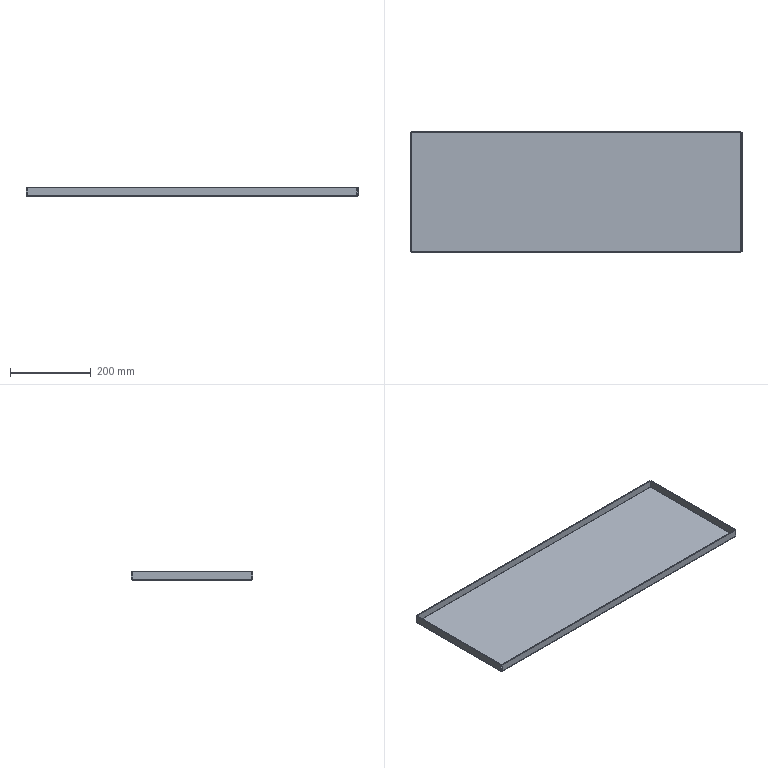Part | STEP file | Part 12 | 1 solid | 38 faces | box 820 x 300 x 20 mm | volume 568950 mm3 | plane 22 | spline 8 | cylinder 8 | commonest cylinder face diameters 1 x4 5 x4
STEP:
#1=CARTESIAN_POINT('',(-407.5,-147.5,-2.));
#2=VERTEX_POINT('',#1);
#3=CARTESIAN_POINT('',(-407.5,147.5,-2.));
#4=VERTEX_POINT('',#3);
#5=CARTESIAN_POINT('',(-407.5,-147.5,-2.));
#6=DIRECTION('',(0.,1.,0.));
#7=VECTOR('',#6,1000.);
#8=LINE('',#5,#7);
#9=EDGE_CURVE('',#2,#4,#8,.T.);
#10=ORIENTED_EDGE('',*,*,#9,.T.);
#11=CARTESIAN_POINT('',(407.5,147.5,-2.));
#12=VERTEX_POINT('',#11);
#13=CARTESIAN_POINT('',(-407.5,147.5,-2.));
#14=DIRECTION('',(1.,0.,0.));
#15=VECTOR('',#14,1000.);
#16=LINE('',#13,#15);
#17=EDGE_CURVE('',#4,#12,#16,.T.);
#18=ORIENTED_EDGE('',*,*,#17,.T.);
#19=CARTESIAN_POINT('',(407.5,-147.5,-2.));
#20=VERTEX_POINT('',#19);
#21=CARTESIAN_POINT('',(407.5,147.5,-2.));
#22=DIRECTION('',(0.,-1.,0.));
#23=VECTOR('',#22,1000.);
#24=LINE('',#21,#23);
#25=EDGE_CURVE('',#12,#20,#24,.T.);
#26=ORIENTED_EDGE('',*,*,#25,.T.);
#27=CARTESIAN_POINT('',(407.5,-147.5,-2.));
#28=DIRECTION('',(-1.,0.,0.));
#29=VECTOR('',#28,1000.);
#30=LINE('',#27,#29);
#31=EDGE_CURVE('',#20,#2,#30,.T.);
#32=ORIENTED_EDGE('',*,*,#31,.T.);
#33=EDGE_LOOP('',(#10,#18,#26,#32));
#34=FACE_OUTER_BOUND('',#33,.T.);
#35=CARTESIAN_POINT('',(0.,0.,-2.));
#36=DIRECTION('',(0.,0.,1.));
#37=DIRECTION('',(1.,0.,0.));
#38=AXIS2_PLACEMENT_3D('',#35,#36,#37);
#39=PLANE('',#38);
#40=ADVANCED_FACE('',(#34),#39,.F.);
#41=CARTESIAN_POINT('',(-407.5,147.5,0.));
#42=VERTEX_POINT('',#41);
#43=CARTESIAN_POINT('',(407.5,147.5,0.));
#44=VERTEX_POINT('',#43);
#45=CARTESIAN_POINT('',(-407.5,147.5,0.));
#46=DIRECTION('',(1.,0.,0.));
#47=VECTOR('',#46,1000.);
#48=LINE('',#45,#47);
#49=EDGE_CURVE('',#42,#44,#48,.T.);
#50=ORIENTED_EDGE('',*,*,#49,.F.);
#51=CARTESIAN_POINT('',(-407.5,-147.5,0.));
#52=VERTEX_POINT('',#51);
#53=CARTESIAN_POINT('',(-407.5,-147.5,0.));
#54=DIRECTION('',(0.,1.,0.));
#55=VECTOR('',#54,1000.);
#56=LINE('',#53,#55);
#57=EDGE_CURVE('',#52,#42,#56,.T.);
#58=ORIENTED_EDGE('',*,*,#57,.F.);
#59=CARTESIAN_POINT('',(407.5,-147.5,0.));
#60=VERTEX_POINT('',#59);
#61=CARTESIAN_POINT('',(407.5,-147.5,0.));
#62=DIRECTION('',(-1.,0.,0.));
#63=VECTOR('',#62,1000.);
#64=LINE('',#61,#63);
#65=EDGE_CURVE('',#60,#52,#64,.T.);
#66=ORIENTED_EDGE('',*,*,#65,.F.);
#67=CARTESIAN_POINT('',(407.5,147.5,0.));
#68=DIRECTION('',(0.,-1.,0.));
#69=VECTOR('',#68,1000.);
#70=LINE('',#67,#69);
#71=EDGE_CURVE('',#44,#60,#70,.T.);
#72=ORIENTED_EDGE('',*,*,#71,.F.);
#73=EDGE_LOOP('',(#50,#58,#66,#72));
#74=FACE_OUTER_BOUND('',#73,.T.);
#75=CARTESIAN_POINT('',(0.,0.,0.));
#76=DIRECTION('',(0.,0.,1.));
#77=DIRECTION('',(1.,0.,0.));
#78=AXIS2_PLACEMENT_3D('',#75,#76,#77);
#79=PLANE('',#78);
#80=ADVANCED_FACE('',(#74),#79,.T.);
#81=CARTESIAN_POINT('',(407.293,150.,0.5));
#82=VERTEX_POINT('',#81);
#83=CARTESIAN_POINT('',(407.293,148.,0.5));
#84=VERTEX_POINT('',#83);
#85=CARTESIAN_POINT('',(407.293,148.,0.5));
#86=DIRECTION('',(0.,-1.,0.));
#87=VECTOR('',#86,1000.);
#88=LINE('',#85,#87);
#89=EDGE_CURVE('',#82,#84,#88,.T.);
#90=ORIENTED_EDGE('',*,*,#89,.T.);
#91=CARTESIAN_POINT('',(407.5,147.5,0.));
#92=CARTESIAN_POINT('',(407.465,147.631,0.));
#93=CARTESIAN_POINT('',(407.431,147.761,0.05389));
#94=CARTESIAN_POINT('',(407.362,147.946,0.239));
#95=CARTESIAN_POINT('',(407.327,148.,0.3691));
#96=CARTESIAN_POINT('',(407.293,148.,0.5));
#97=B_SPLINE_CURVE_WITH_KNOTS('',3,(#91,#92,#93,#94,#95,#96),.UNSPECIFIED.,.F.,.F.,(4,2,4),(0.,0.5,1.),.UNSPECIFIED.);
#98=EDGE_CURVE('',#44,#84,#97,.T.);
#99=ORIENTED_EDGE('',*,*,#98,.F.);
#100=CARTESIAN_POINT('',(407.5,147.5,0.));
#101=DIRECTION('',(0.,0.,-1.));
#102=VECTOR('',#101,1000.);
#103=LINE('',#100,#102);
#104=EDGE_CURVE('',#44,#12,#103,.T.);
#105=ORIENTED_EDGE('',*,*,#104,.T.);
#106=CARTESIAN_POINT('',(407.5,147.5,-2.));
#107=CARTESIAN_POINT('',(407.483,147.827,-2.));
#108=CARTESIAN_POINT('',(407.465,148.154,-1.935));
#109=CARTESIAN_POINT('',(407.431,148.759,-1.684));
#110=CARTESIAN_POINT('',(407.414,149.036,-1.499));
#111=CARTESIAN_POINT('',(407.379,149.499,-1.036));
#112=CARTESIAN_POINT('',(407.362,149.684,-0.759));
#113=CARTESIAN_POINT('',(407.327,149.935,-0.1544));
#114=CARTESIAN_POINT('',(407.31,150.,0.1728));
#115=CARTESIAN_POINT('',(407.293,150.,0.5));
#116=B_SPLINE_CURVE_WITH_KNOTS('',3,(#106,#107,#108,#109,#110,#111,#112,#113,#114,#115),.UNSPECIFIED.,.F.,.F.,(4,2,2,2,4),(0.,0.25,0.5,0.75,1.),.UNSPECIFIED.);
#117=EDGE_CURVE('',#12,#82,#116,.T.);
#118=ORIENTED_EDGE('',*,*,#117,.T.);
#119=EDGE_LOOP('',(#90,#99,#105,#118));
#120=FACE_OUTER_BOUND('',#119,.T.);
#121=CARTESIAN_POINT('',(407.5,147.5,-2.02));
#122=CARTESIAN_POINT('',(407.483,147.83,-2.02));
#123=CARTESIAN_POINT('',(407.465,148.16,-1.954));
#124=CARTESIAN_POINT('',(407.431,148.769,-1.702));
#125=CARTESIAN_POINT('',(407.414,149.049,-1.515));
#126=CARTESIAN_POINT('',(407.379,149.515,-1.049));
#127=CARTESIAN_POINT('',(407.362,149.702,-0.7691));
#128=CARTESIAN_POINT('',(407.327,149.954,-0.1596));
#129=CARTESIAN_POINT('',(407.31,150.02,0.1701));
#130=CARTESIAN_POINT('',(407.293,150.02,0.5));
#131=CARTESIAN_POINT('',(407.5,147.5,-2.));
#132=CARTESIAN_POINT('',(407.483,147.827,-2.));
#133=CARTESIAN_POINT('',(407.465,148.154,-1.935));
#134=CARTESIAN_POINT('',(407.431,148.759,-1.684));
#135=CARTESIAN_POINT('',(407.414,149.036,-1.499));
#136=CARTESIAN_POINT('',(407.379,149.499,-1.036));
#137=CARTESIAN_POINT('',(407.362,149.684,-0.759));
#138=CARTESIAN_POINT('',(407.327,149.935,-0.1544));
#139=CARTESIAN_POINT('',(407.31,150.,0.1727));
#140=CARTESIAN_POINT('',(407.293,150.,0.5));
#141=CARTESIAN_POINT('',(407.5,147.5,0.));
#142=CARTESIAN_POINT('',(407.483,147.565,0.));
#143=CARTESIAN_POINT('',(407.465,147.631,0.01301));
#144=CARTESIAN_POINT('',(407.431,147.752,0.06311));
#145=CARTESIAN_POINT('',(407.414,147.807,0.1002));
#146=CARTESIAN_POINT('',(407.379,147.9,0.1927));
#147=CARTESIAN_POINT('',(407.362,147.937,0.2482));
#148=CARTESIAN_POINT('',(407.327,147.987,0.3691));
#149=CARTESIAN_POINT('',(407.31,148.,0.4345));
#150=CARTESIAN_POINT('',(407.293,148.,0.5));
#151=CARTESIAN_POINT('',(407.5,147.5,0.0202));
#152=CARTESIAN_POINT('',(407.483,147.563,0.0202));
#153=CARTESIAN_POINT('',(407.465,147.626,0.03269));
#154=CARTESIAN_POINT('',(407.431,147.742,0.08076));
#155=CARTESIAN_POINT('',(407.414,147.795,0.1163));
#156=CARTESIAN_POINT('',(407.379,147.884,0.2051));
#157=CARTESIAN_POINT('',(407.362,147.919,0.2584));
#158=CARTESIAN_POINT('',(407.327,147.967,0.3744));
#159=CARTESIAN_POINT('',(407.31,147.98,0.4372));
#160=CARTESIAN_POINT('',(407.293,147.98,0.5));
#161=B_SPLINE_SURFACE_WITH_KNOTS('',1,3,((#121,#122,#123,#124,#125,#126,#127,#128,#129,#130),(#131,#132,#133,#134,#135,#136,#137,#138,#139,#140),(#141,#142,#143,#144,#145,#146,#147,#148,#149,#150),(#151,#152,#153,#154,#155,#156,#157,#158,#159,#160)),.UNSPECIFIED.,.F.,.F.,.F.,(2,1,1,2),(4,2,2,2,4),(-0.01,0.,1.,1.01),(0.,0.25,0.5,0.75,1.),.UNSPECIFIED.);
#162=ADVANCED_FACE('',(#120),#161,.F.);
#163=CARTESIAN_POINT('',(-407.293,148.,0.5));
#164=VERTEX_POINT('',#163);
#165=CARTESIAN_POINT('',(-407.293,148.,0.5));
#166=CARTESIAN_POINT('',(-407.327,148.,0.3691));
#167=CARTESIAN_POINT('',(-407.362,147.946,0.239));
#168=CARTESIAN_POINT('',(-407.431,147.761,0.05389));
#169=CARTESIAN_POINT('',(-407.465,147.631,0.));
#170=CARTESIAN_POINT('',(-407.5,147.5,0.));
#171=B_SPLINE_CURVE_WITH_KNOTS('',3,(#165,#166,#167,#168,#169,#170),.UNSPECIFIED.,.F.,.F.,(4,2,4),(0.,0.5,1.),.UNSPECIFIED.);
#172=EDGE_CURVE('',#164,#42,#171,.T.);
#173=ORIENTED_EDGE('',*,*,#172,.F.);
#174=CARTESIAN_POINT('',(-407.293,150.,0.5));
#175=VERTEX_POINT('',#174);
#176=CARTESIAN_POINT('',(-407.293,148.,0.5));
#177=DIRECTION('',(0.,-1.,0.));
#178=VECTOR('',#177,1000.);
#179=LINE('',#176,#178);
#180=EDGE_CURVE('',#175,#164,#179,.T.);
#181=ORIENTED_EDGE('',*,*,#180,.F.);
#182=CARTESIAN_POINT('',(-407.293,150.,0.5));
#183=CARTESIAN_POINT('',(-407.31,150.,0.1728));
#184=CARTESIAN_POINT('',(-407.327,149.935,-0.1544));
#185=CARTESIAN_POINT('',(-407.362,149.684,-0.759));
#186=CARTESIAN_POINT('',(-407.379,149.499,-1.036));
#187=CARTESIAN_POINT('',(-407.414,149.036,-1.499));
#188=CARTESIAN_POINT('',(-407.431,148.759,-1.684));
#189=CARTESIAN_POINT('',(-407.465,148.154,-1.935));
#190=CARTESIAN_POINT('',(-407.483,147.827,-2.));
#191=CARTESIAN_POINT('',(-407.5,147.5,-2.));
#192=B_SPLINE_CURVE_WITH_KNOTS('',3,(#182,#183,#184,#185,#186,#187,#188,#189,#190,#191),.UNSPECIFIED.,.F.,.F.,(4,2,2,2,4),(0.,0.25,0.5,0.75,1.),.UNSPECIFIED.);
#193=EDGE_CURVE('',#175,#4,#192,.T.);
#194=ORIENTED_EDGE('',*,*,#193,.T.);
#195=CARTESIAN_POINT('',(-407.5,147.5,0.));
#196=DIRECTION('',(0.,0.,-1.));
#197=VECTOR('',#196,1000.);
#198=LINE('',#195,#197);
#199=EDGE_CURVE('',#42,#4,#198,.T.);
#200=ORIENTED_EDGE('',*,*,#199,.F.);
#201=EDGE_LOOP('',(#173,#181,#194,#200));
#202=FACE_OUTER_BOUND('',#201,.T.);
#203=CARTESIAN_POINT('',(-407.293,150.02,0.5));
#204=CARTESIAN_POINT('',(-407.31,150.02,0.1701));
#205=CARTESIAN_POINT('',(-407.327,149.954,-0.1596));
#206=CARTESIAN_POINT('',(-407.362,149.702,-0.7691));
#207=CARTESIAN_POINT('',(-407.379,149.515,-1.049));
#208=CARTESIAN_POINT('',(-407.414,149.049,-1.515));
#209=CARTESIAN_POINT('',(-407.431,148.769,-1.702));
#210=CARTESIAN_POINT('',(-407.465,148.16,-1.954));
#211=CARTESIAN_POINT('',(-407.483,147.83,-2.02));
#212=CARTESIAN_POINT('',(-407.5,147.5,-2.02));
#213=CARTESIAN_POINT('',(-407.293,150.,0.5));
#214=CARTESIAN_POINT('',(-407.31,150.,0.1727));
#215=CARTESIAN_POINT('',(-407.327,149.935,-0.1544));
#216=CARTESIAN_POINT('',(-407.362,149.684,-0.759));
#217=CARTESIAN_POINT('',(-407.379,149.499,-1.036));
#218=CARTESIAN_POINT('',(-407.414,149.036,-1.499));
#219=CARTESIAN_POINT('',(-407.431,148.759,-1.684));
#220=CARTESIAN_POINT('',(-407.465,148.154,-1.935));
#221=CARTESIAN_POINT('',(-407.483,147.827,-2.));
#222=CARTESIAN_POINT('',(-407.5,147.5,-2.));
#223=CARTESIAN_POINT('',(-407.293,148.,0.5));
#224=CARTESIAN_POINT('',(-407.31,148.,0.4345));
#225=CARTESIAN_POINT('',(-407.327,147.987,0.3691));
#226=CARTESIAN_POINT('',(-407.362,147.937,0.2482));
#227=CARTESIAN_POINT('',(-407.379,147.9,0.1927));
#228=CARTESIAN_POINT('',(-407.414,147.807,0.1002));
#229=CARTESIAN_POINT('',(-407.431,147.752,0.06311));
#230=CARTESIAN_POINT('',(-407.465,147.631,0.01301));
#231=CARTESIAN_POINT('',(-407.483,147.565,0.));
#232=CARTESIAN_POINT('',(-407.5,147.5,0.));
#233=CARTESIAN_POINT('',(-407.293,147.98,0.5));
#234=CARTESIAN_POINT('',(-407.31,147.98,0.4372));
#235=CARTESIAN_POINT('',(-407.327,147.967,0.3744));
#236=CARTESIAN_POINT('',(-407.362,147.919,0.2584));
#237=CARTESIAN_POINT('',(-407.379,147.884,0.2051));
#238=CARTESIAN_POINT('',(-407.414,147.795,0.1163));
#239=CARTESIAN_POINT('',(-407.431,147.742,0.08076));
#240=CARTESIAN_POINT('',(-407.465,147.626,0.03269));
#241=CARTESIAN_POINT('',(-407.483,147.563,0.0202));
#242=CARTESIAN_POINT('',(-407.5,147.5,0.0202));
#243=B_SPLINE_SURFACE_WITH_KNOTS('',1,3,((#203,#204,#205,#206,#207,#208,#209,#210,#211,#212),(#213,#214,#215,#216,#217,#218,#219,#220,#221,#222),(#223,#224,#225,#226,#227,#228,#229,#230,#231,#232),(#233,#234,#235,#236,#237,#238,#239,#240,#241,#242)),.UNSPECIFIED.,.F.,.F.,.F.,(2,1,1,2),(4,2,2,2,4),(-0.01,0.,1.,1.01),(0.,0.25,0.5,0.75,1.),.UNSPECIFIED.);
#244=ADVANCED_FACE('',(#202),#243,.F.);
#245=ORIENTED_EDGE('',*,*,#17,.F.);
#246=ORIENTED_EDGE('',*,*,#193,.F.);
#247=CARTESIAN_POINT('',(0.,150.,0.5));
#248=DIRECTION('',(-1.,0.,0.));
#249=VECTOR('',#248,1000.);
#250=LINE('',#247,#249);
#251=EDGE_CURVE('',#82,#175,#250,.T.);
#252=ORIENTED_EDGE('',*,*,#251,.F.);
#253=ORIENTED_EDGE('',*,*,#117,.F.);
#254=EDGE_LOOP('',(#245,#246,#252,#253));
#255=FACE_OUTER_BOUND('',#254,.T.);
#256=CARTESIAN_POINT('',(-407.5,147.5,0.5));
#257=DIRECTION('',(-1.,0.,0.));
#258=DIRECTION('',(0.,1.,0.));
#259=AXIS2_PLACEMENT_3D('',#256,#257,#258);
#260=CYLINDRICAL_SURFACE('',#259,2.5);
#261=ADVANCED_FACE('',(#255),#260,.T.);
#262=ORIENTED_EDGE('',*,*,#49,.T.);
#263=ORIENTED_EDGE('',*,*,#98,.T.);
#264=CARTESIAN_POINT('',(410.,148.,0.5));
#265=DIRECTION('',(-1.,0.,0.));
#266=VECTOR('',#265,1000.);
#267=LINE('',#264,#266);
#268=EDGE_CURVE('',#84,#164,#267,.T.);
#269=ORIENTED_EDGE('',*,*,#268,.T.);
#270=ORIENTED_EDGE('',*,*,#172,.T.);
#271=EDGE_LOOP('',(#262,#263,#269,#270));
#272=FACE_OUTER_BOUND('',#271,.T.);
#273=CARTESIAN_POINT('',(-407.5,147.5,0.5));
#274=DIRECTION('',(-1.,0.,0.));
#275=DIRECTION('',(0.,1.,0.));
#276=AXIS2_PLACEMENT_3D('',#273,#274,#275);
#277=CYLINDRICAL_SURFACE('',#276,0.5);
#278=ADVANCED_FACE('',(#272),#277,.F.);
#279=CARTESIAN_POINT('',(407.293,148.,18.));
#280=VERTEX_POINT('',#279);
#281=CARTESIAN_POINT('',(407.293,150.,18.));
#282=VERTEX_POINT('',#281);
#283=CARTESIAN_POINT('',(407.293,150.,18.));
#284=DIRECTION('',(0.,1.,0.));
#285=VECTOR('',#284,1000.);
#286=LINE('',#283,#285);
#287=EDGE_CURVE('',#280,#282,#286,.T.);
#288=ORIENTED_EDGE('',*,*,#287,.F.);
#289=CARTESIAN_POINT('',(407.293,148.,0.));
#290=DIRECTION('',(0.,0.,1.));
#291=VECTOR('',#290,1000.);
#292=LINE('',#289,#291);
#293=EDGE_CURVE('',#84,#280,#292,.T.);
#294=ORIENTED_EDGE('',*,*,#293,.F.);
#295=ORIENTED_EDGE('',*,*,#89,.F.);
#296=CARTESIAN_POINT('',(407.293,150.,0.));
#297=DIRECTION('',(0.,0.,-1.));
#298=VECTOR('',#297,1000.);
#299=LINE('',#296,#298);
#300=EDGE_CURVE('',#282,#82,#299,.T.);
#301=ORIENTED_EDGE('',*,*,#300,.F.);
#302=EDGE_LOOP('',(#288,#294,#295,#301));
#303=FACE_OUTER_BOUND('',#302,.T.);
#304=CARTESIAN_POINT('',(407.293,148.,0.));
#305=DIRECTION('',(1.,0.,0.));
#306=DIRECTION('',(0.,0.,-1.));
#307=AXIS2_PLACEMENT_3D('',#304,#305,#306);
#308=PLANE('',#307);
#309=ADVANCED_FACE('',(#303),#308,.T.);
#310=CARTESIAN_POINT('',(-407.293,150.,18.));
#311=VERTEX_POINT('',#310);
#312=CARTESIAN_POINT('',(-407.293,150.,0.));
#313=DIRECTION('',(0.,0.,-1.));
#314=VECTOR('',#313,1000.);
#315=LINE('',#312,#314);
#316=EDGE_CURVE('',#311,#175,#315,.T.);
#317=ORIENTED_EDGE('',*,*,#316,.F.);
#318=CARTESIAN_POINT('',(-410.,150.,18.));
#319=DIRECTION('',(-1.,0.,0.));
#320=VECTOR('',#319,1000.);
#321=LINE('',#318,#320);
#322=EDGE_CURVE('',#282,#311,#321,.T.);
#323=ORIENTED_EDGE('',*,*,#322,.F.);
#324=ORIENTED_EDGE('',*,*,#300,.T.);
#325=ORIENTED_EDGE('',*,*,#251,.T.);
#326=EDGE_LOOP('',(#317,#323,#324,#325));
#327=FACE_OUTER_BOUND('',#326,.T.);
#328=CARTESIAN_POINT('',(0.,150.,0.));
#329=DIRECTION('',(0.,1.,0.));
#330=DIRECTION('',(0.,0.,1.));
#331=AXIS2_PLACEMENT_3D('',#328,#329,#330);
#332=PLANE('',#331);
#333=ADVANCED_FACE('',(#327),#332,.T.);
#334=CARTESIAN_POINT('',(-407.293,148.,18.));
#335=VERTEX_POINT('',#334);
#336=CARTESIAN_POINT('',(0.,148.,18.));
#337=DIRECTION('',(-1.,0.,0.));
#338=VECTOR('',#337,1000.);
#339=LINE('',#336,#338);
#340=EDGE_CURVE('',#280,#335,#339,.T.);
#341=ORIENTED_EDGE('',*,*,#340,.T.);
#342=CARTESIAN_POINT('',(-407.293,148.,0.));
#343=DIRECTION('',(0.,0.,1.));
#344=VECTOR('',#343,1000.);
#345=LINE('',#342,#344);
#346=EDGE_CURVE('',#164,#335,#345,.T.);
#347=ORIENTED_EDGE('',*,*,#346,.F.);
#348=ORIENTED_EDGE('',*,*,#268,.F.);
#349=ORIENTED_EDGE('',*,*,#293,.T.);
#350=EDGE_LOOP('',(#341,#347,#348,#349));
#351=FACE_OUTER_BOUND('',#350,.T.);
#352=CARTESIAN_POINT('',(0.,148.,0.));
#353=DIRECTION('',(0.,1.,0.));
#354=DIRECTION('',(0.,0.,1.));
#355=AXIS2_PLACEMENT_3D('',#352,#353,#354);
#356=PLANE('',#355);
#357=ADVANCED_FACE('',(#351),#356,.F.);
#358=CARTESIAN_POINT('',(-407.293,148.,18.));
#359=DIRECTION('',(0.,1.,0.));
#360=VECTOR('',#359,1000.);
#361=LINE('',#358,#360);
#362=EDGE_CURVE('',#335,#311,#361,.T.);
#363=ORIENTED_EDGE('',*,*,#362,.F.);
#364=ORIENTED_EDGE('',*,*,#340,.F.);
#365=ORIENTED_EDGE('',*,*,#287,.T.);
#366=ORIENTED_EDGE('',*,*,#322,.T.);
#367=EDGE_LOOP('',(#363,#364,#365,#366));
#368=FACE_OUTER_BOUND('',#367,.T.);
#369=CARTESIAN_POINT('',(-410.,150.,18.));
#370=DIRECTION('',(0.,0.,1.));
#371=DIRECTION('',(0.,-1.,0.));
#372=AXIS2_PLACEMENT_3D('',#369,#370,#371);
#373=PLANE('',#372);
#374=ADVANCED_FACE('',(#368),#373,.T.);
#375=ORIENTED_EDGE('',*,*,#346,.T.);
#376=ORIENTED_EDGE('',*,*,#362,.T.);
#377=ORIENTED_EDGE('',*,*,#316,.T.);
#378=ORIENTED_EDGE('',*,*,#180,.T.);
#379=EDGE_LOOP('',(#375,#376,#377,#378));
#380=FACE_OUTER_BOUND('',#379,.T.);
#381=CARTESIAN_POINT('',(-407.293,148.,0.));
#382=DIRECTION('',(1.,0.,0.));
#383=DIRECTION('',(0.,0.,-1.));
#384=AXIS2_PLACEMENT_3D('',#381,#382,#383);
#385=PLANE('',#384);
#386=ADVANCED_FACE('',(#380),#385,.F.);
#387=CARTESIAN_POINT('',(410.,-147.293,0.5));
#388=VERTEX_POINT('',#387);
#389=CARTESIAN_POINT('',(408.,-147.293,0.5));
#390=VERTEX_POINT('',#389);
#391=CARTESIAN_POINT('',(408.,-147.293,0.5));
#392=DIRECTION('',(-1.,0.,0.));
#393=VECTOR('',#392,1000.);
#394=LINE('',#391,#393);
#395=EDGE_CURVE('',#388,#390,#394,.T.);
#396=ORIENTED_EDGE('',*,*,#395,.T.);
#397=CARTESIAN_POINT('',(407.5,-147.5,0.));
#398=CARTESIAN_POINT('',(407.631,-147.465,0.));
#399=CARTESIAN_POINT('',(407.761,-147.431,0.05389));
#400=CARTESIAN_POINT('',(407.946,-147.362,0.239));
#401=CARTESIAN_POINT('',(408.,-147.327,0.3691));
#402=CARTESIAN_POINT('',(408.,-147.293,0.5));
#403=B_SPLINE_CURVE_WITH_KNOTS('',3,(#397,#398,#399,#400,#401,#402),.UNSPECIFIED.,.F.,.F.,(4,2,4),(0.,0.5,1.),.UNSPECIFIED.);
#404=EDGE_CURVE('',#60,#390,#403,.T.);
#405=ORIENTED_EDGE('',*,*,#404,.F.);
#406=CARTESIAN_POINT('',(407.5,-147.5,0.));
#407=DIRECTION('',(0.,0.,-1.));
#408=VECTOR('',#407,1000.);
#409=LINE('',#406,#408);
#410=EDGE_CURVE('',#60,#20,#409,.T.);
#411=ORIENTED_EDGE('',*,*,#410,.T.);
#412=CARTESIAN_POINT('',(407.5,-147.5,-2.));
#413=CARTESIAN_POINT('',(407.827,-147.483,-2.));
#414=CARTESIAN_POINT('',(408.154,-147.465,-1.935));
#415=CARTESIAN_POINT('',(408.759,-147.431,-1.684));
#416=CARTESIAN_POINT('',(409.036,-147.414,-1.499));
#417=CARTESIAN_POINT('',(409.499,-147.379,-1.036));
#418=CARTESIAN_POINT('',(409.684,-147.362,-0.759));
#419=CARTESIAN_POINT('',(409.935,-147.327,-0.1544));
#420=CARTESIAN_POINT('',(410.,-147.31,0.1728));
#421=CARTESIAN_POINT('',(410.,-147.293,0.5));
#422=B_SPLINE_CURVE_WITH_KNOTS('',3,(#412,#413,#414,#415,#416,#417,#418,#419,#420,#421),.UNSPECIFIED.,.F.,.F.,(4,2,2,2,4),(0.,0.25,0.5,0.75,1.),.UNSPECIFIED.);
#423=EDGE_CURVE('',#20,#388,#422,.T.);
#424=ORIENTED_EDGE('',*,*,#423,.T.);
#425=EDGE_LOOP('',(#396,#405,#411,#424));
#426=FACE_OUTER_BOUND('',#425,.T.);
#427=CARTESIAN_POINT('',(407.5,-147.5,-2.02));
#428=CARTESIAN_POINT('',(407.83,-147.483,-2.02));
#429=CARTESIAN_POINT('',(408.16,-147.465,-1.954));
#430=CARTESIAN_POINT('',(408.769,-147.431,-1.702));
#431=CARTESIAN_POINT('',(409.049,-147.414,-1.515));
#432=CARTESIAN_POINT('',(409.515,-147.379,-1.049));
#433=CARTESIAN_POINT('',(409.702,-147.362,-0.7691));
#434=CARTESIAN_POINT('',(409.954,-147.327,-0.1596));
#435=CARTESIAN_POINT('',(410.02,-147.31,0.1701));
#436=CARTESIAN_POINT('',(410.02,-147.293,0.5));
#437=CARTESIAN_POINT('',(407.5,-147.5,-2.));
#438=CARTESIAN_POINT('',(407.827,-147.483,-2.));
#439=CARTESIAN_POINT('',(408.154,-147.465,-1.935));
#440=CARTESIAN_POINT('',(408.759,-147.431,-1.684));
#441=CARTESIAN_POINT('',(409.036,-147.414,-1.499));
#442=CARTESIAN_POINT('',(409.499,-147.379,-1.036));
#443=CARTESIAN_POINT('',(409.684,-147.362,-0.759));
#444=CARTESIAN_POINT('',(409.935,-147.327,-0.1544));
#445=CARTESIAN_POINT('',(410.,-147.31,0.1727));
#446=CARTESIAN_POINT('',(410.,-147.293,0.5));
#447=CARTESIAN_POINT('',(407.5,-147.5,0.));
#448=CARTESIAN_POINT('',(407.565,-147.483,0.));
#449=CARTESIAN_POINT('',(407.631,-147.465,0.01301));
#450=CARTESIAN_POINT('',(407.752,-147.431,0.06311));
#451=CARTESIAN_POINT('',(407.807,-147.414,0.1002));
#452=CARTESIAN_POINT('',(407.9,-147.379,0.1927));
#453=CARTESIAN_POINT('',(407.937,-147.362,0.2482));
#454=CARTESIAN_POINT('',(407.987,-147.327,0.3691));
#455=CARTESIAN_POINT('',(408.,-147.31,0.4345));
#456=CARTESIAN_POINT('',(408.,-147.293,0.5));
#457=CARTESIAN_POINT('',(407.5,-147.5,0.0202));
#458=CARTESIAN_POINT('',(407.563,-147.483,0.0202));
#459=CARTESIAN_POINT('',(407.626,-147.465,0.03269));
#460=CARTESIAN_POINT('',(407.742,-147.431,0.08076));
#461=CARTESIAN_POINT('',(407.795,-147.414,0.1163));
#462=CARTESIAN_POINT('',(407.884,-147.379,0.2051));
#463=CARTESIAN_POINT('',(407.919,-147.362,0.2584));
#464=CARTESIAN_POINT('',(407.967,-147.327,0.3744));
#465=CARTESIAN_POINT('',(407.98,-147.31,0.4372));
#466=CARTESIAN_POINT('',(407.98,-147.293,0.5));
#467=B_SPLINE_SURFACE_WITH_KNOTS('',1,3,((#427,#428,#429,#430,#431,#432,#433,#434,#435,#436),(#437,#438,#439,#440,#441,#442,#443,#444,#445,#446),(#447,#448,#449,#450,#451,#452,#453,#454,#455,#456),(#457,#458,#459,#460,#461,#462,#463,#464,#465,#466)),.UNSPECIFIED.,.F.,.F.,.F.,(2,1,1,2),(4,2,2,2,4),(-0.01,0.,1.,1.01),(0.,0.25,0.5,0.75,1.),.UNSPECIFIED.);
#468=ADVANCED_FACE('',(#426),#467,.F.);
#469=CARTESIAN_POINT('',(408.,147.293,0.5));
#470=VERTEX_POINT('',#469);
#471=CARTESIAN_POINT('',(408.,147.293,0.5));
#472=CARTESIAN_POINT('',(408.,147.327,0.3691));
#473=CARTESIAN_POINT('',(407.946,147.362,0.239));
#474=CARTESIAN_POINT('',(407.761,147.431,0.05389));
#475=CARTESIAN_POINT('',(407.631,147.465,0.));
#476=CARTESIAN_POINT('',(407.5,147.5,0.));
#477=B_SPLINE_CURVE_WITH_KNOTS('',3,(#471,#472,#473,#474,#475,#476),.UNSPECIFIED.,.F.,.F.,(4,2,4),(0.,0.5,1.),.UNSPECIFIED.);
#478=EDGE_CURVE('',#470,#44,#477,.T.);
#479=ORIENTED_EDGE('',*,*,#478,.F.);
#480=CARTESIAN_POINT('',(410.,147.293,0.5));
#481=VERTEX_POINT('',#480);
#482=CARTESIAN_POINT('',(408.,147.293,0.5));
#483=DIRECTION('',(-1.,0.,0.));
#484=VECTOR('',#483,1000.);
#485=LINE('',#482,#484);
#486=EDGE_CURVE('',#481,#470,#485,.T.);
#487=ORIENTED_EDGE('',*,*,#486,.F.);
#488=CARTESIAN_POINT('',(410.,147.293,0.5));
#489=CARTESIAN_POINT('',(410.,147.31,0.1728));
#490=CARTESIAN_POINT('',(409.935,147.327,-0.1544));
#491=CARTESIAN_POINT('',(409.684,147.362,-0.759));
#492=CARTESIAN_POINT('',(409.499,147.379,-1.036));
#493=CARTESIAN_POINT('',(409.036,147.414,-1.499));
#494=CARTESIAN_POINT('',(408.759,147.431,-1.684));
#495=CARTESIAN_POINT('',(408.154,147.465,-1.935));
#496=CARTESIAN_POINT('',(407.827,147.483,-2.));
#497=CARTESIAN_POINT('',(407.5,147.5,-2.));
#498=B_SPLINE_CURVE_WITH_KNOTS('',3,(#488,#489,#490,#491,#492,#493,#494,#495,#496,#497),.UNSPECIFIED.,.F.,.F.,(4,2,2,2,4),(0.,0.25,0.5,0.75,1.),.UNSPECIFIED.);
#499=EDGE_CURVE('',#481,#12,#498,.T.);
#500=ORIENTED_EDGE('',*,*,#499,.T.);
#501=ORIENTED_EDGE('',*,*,#104,.F.);
#502=EDGE_LOOP('',(#479,#487,#500,#501));
#503=FACE_OUTER_BOUND('',#502,.T.);
#504=CARTESIAN_POINT('',(410.02,147.293,0.5));
#505=CARTESIAN_POINT('',(410.02,147.31,0.1701));
#506=CARTESIAN_POINT('',(409.954,147.327,-0.1596));
#507=CARTESIAN_POINT('',(409.702,147.362,-0.7691));
#508=CARTESIAN_POINT('',(409.515,147.379,-1.049));
#509=CARTESIAN_POINT('',(409.049,147.414,-1.515));
#510=CARTESIAN_POINT('',(408.769,147.431,-1.702));
#511=CARTESIAN_POINT('',(408.16,147.465,-1.954));
#512=CARTESIAN_POINT('',(407.83,147.483,-2.02));
#513=CARTESIAN_POINT('',(407.5,147.5,-2.02));
#514=CARTESIAN_POINT('',(410.,147.293,0.5));
#515=CARTESIAN_POINT('',(410.,147.31,0.1727));
#516=CARTESIAN_POINT('',(409.935,147.327,-0.1544));
#517=CARTESIAN_POINT('',(409.684,147.362,-0.759));
#518=CARTESIAN_POINT('',(409.499,147.379,-1.036));
#519=CARTESIAN_POINT('',(409.036,147.414,-1.499));
#520=CARTESIAN_POINT('',(408.759,147.431,-1.684));
#521=CARTESIAN_POINT('',(408.154,147.465,-1.935));
#522=CARTESIAN_POINT('',(407.827,147.483,-2.));
#523=CARTESIAN_POINT('',(407.5,147.5,-2.));
#524=CARTESIAN_POINT('',(408.,147.293,0.5));
#525=CARTESIAN_POINT('',(408.,147.31,0.4345));
#526=CARTESIAN_POINT('',(407.987,147.327,0.3691));
#527=CARTESIAN_POINT('',(407.937,147.362,0.2482));
#528=CARTESIAN_POINT('',(407.9,147.379,0.1927));
#529=CARTESIAN_POINT('',(407.807,147.414,0.1002));
#530=CARTESIAN_POINT('',(407.752,147.431,0.06311));
#531=CARTESIAN_POINT('',(407.631,147.465,0.01301));
#532=CARTESIAN_POINT('',(407.565,147.483,0.));
#533=CARTESIAN_POINT('',(407.5,147.5,0.));
#534=CARTESIAN_POINT('',(407.98,147.293,0.5));
#535=CARTESIAN_POINT('',(407.98,147.31,0.4372));
#536=CARTESIAN_POINT('',(407.967,147.327,0.3744));
#537=CARTESIAN_POINT('',(407.919,147.362,0.2584));
#538=CARTESIAN_POINT('',(407.884,147.379,0.2051));
#539=CARTESIAN_POINT('',(407.795,147.414,0.1163));
#540=CARTESIAN_POINT('',(407.742,147.431,0.08076));
#541=CARTESIAN_POINT('',(407.626,147.465,0.03269));
#542=CARTESIAN_POINT('',(407.563,147.483,0.0202));
#543=CARTESIAN_POINT('',(407.5,147.5,0.0202));
#544=B_SPLINE_SURFACE_WITH_KNOTS('',1,3,((#504,#505,#506,#507,#508,#509,#510,#511,#512,#513),(#514,#515,#516,#517,#518,#519,#520,#521,#522,#523),(#524,#525,#526,#527,#528,#529,#530,#531,#532,#533),(#534,#535,#536,#537,#538,#539,#540,#541,#542,#543)),.UNSPECIFIED.,.F.,.F.,.F.,(2,1,1,2),(4,2,2,2,4),(-0.01,0.,1.,1.01),(0.,0.25,0.5,0.75,1.),.UNSPECIFIED.);
#545=ADVANCED_FACE('',(#503),#544,.F.);
#546=ORIENTED_EDGE('',*,*,#25,.F.);
#547=ORIENTED_EDGE('',*,*,#499,.F.);
#548=CARTESIAN_POINT('',(410.,-150.,0.5));
#549=DIRECTION('',(0.,-1.,0.));
#550=VECTOR('',#549,1000.);
#551=LINE('',#548,#550);
#552=EDGE_CURVE('',#481,#388,#551,.T.);
#553=ORIENTED_EDGE('',*,*,#552,.T.);
#554=ORIENTED_EDGE('',*,*,#423,.F.);
#555=EDGE_LOOP('',(#546,#547,#553,#554));
#556=FACE_OUTER_BOUND('',#555,.T.);
#557=CARTESIAN_POINT('',(407.5,147.5,0.5));
#558=DIRECTION('',(0.,1.,0.));
#559=DIRECTION('',(1.,0.,0.));
#560=AXIS2_PLACEMENT_3D('',#557,#558,#559);
#561=CYLINDRICAL_SURFACE('',#560,2.5);
#562=ADVANCED_FACE('',(#556),#561,.T.);
#563=ORIENTED_EDGE('',*,*,#71,.T.);
#564=ORIENTED_EDGE('',*,*,#404,.T.);
#565=CARTESIAN_POINT('',(408.,-150.,0.5));
#566=DIRECTION('',(0.,1.,0.));
#567=VECTOR('',#566,1000.);
#568=LINE('',#565,#567);
#569=EDGE_CURVE('',#390,#470,#568,.T.);
#570=ORIENTED_EDGE('',*,*,#569,.T.);
#571=ORIENTED_EDGE('',*,*,#478,.T.);
#572=EDGE_LOOP('',(#563,#564,#570,#571));
#573=FACE_OUTER_BOUND('',#572,.T.);
#574=CARTESIAN_POINT('',(407.5,147.5,0.5));
#575=DIRECTION('',(0.,1.,0.));
#576=DIRECTION('',(1.,0.,0.));
#577=AXIS2_PLACEMENT_3D('',#574,#575,#576);
#578=CYLINDRICAL_SURFACE('',#577,0.5);
#579=ADVANCED_FACE('',(#573),#578,.F.);
#580=CARTESIAN_POINT('',(408.,-147.293,18.));
#581=VERTEX_POINT('',#580);
#582=CARTESIAN_POINT('',(410.,-147.293,18.));
#583=VERTEX_POINT('',#582);
#584=CARTESIAN_POINT('',(410.,-147.293,18.));
#585=DIRECTION('',(1.,0.,0.));
#586=VECTOR('',#585,1000.);
#587=LINE('',#584,#586);
#588=EDGE_CURVE('',#581,#583,#587,.T.);
#589=ORIENTED_EDGE('',*,*,#588,.F.);
#590=CARTESIAN_POINT('',(408.,-147.293,0.));
#591=DIRECTION('',(0.,0.,1.));
#592=VECTOR('',#591,1000.);
#593=LINE('',#590,#592);
#594=EDGE_CURVE('',#390,#581,#593,.T.);
#595=ORIENTED_EDGE('',*,*,#594,.F.);
#596=ORIENTED_EDGE('',*,*,#395,.F.);
#597=CARTESIAN_POINT('',(410.,-147.293,0.));
#598=DIRECTION('',(0.,0.,1.));
#599=VECTOR('',#598,1000.);
#600=LINE('',#597,#599);
#601=EDGE_CURVE('',#388,#583,#600,.T.);
#602=ORIENTED_EDGE('',*,*,#601,.T.);
#603=EDGE_LOOP('',(#589,#595,#596,#602));
#604=FACE_OUTER_BOUND('',#603,.T.);
#605=CARTESIAN_POINT('',(408.,-147.293,0.));
#606=DIRECTION('',(0.,-1.,0.));
#607=DIRECTION('',(0.,0.,-1.));
#608=AXIS2_PLACEMENT_3D('',#605,#606,#607);
#609=PLANE('',#608);
#610=ADVANCED_FACE('',(#604),#609,.T.);
#611=ORIENTED_EDGE('',*,*,#552,.F.);
#612=CARTESIAN_POINT('',(410.,147.293,18.));
#613=VERTEX_POINT('',#612);
#614=CARTESIAN_POINT('',(410.,147.293,0.));
#615=DIRECTION('',(0.,0.,1.));
#616=VECTOR('',#615,1000.);
#617=LINE('',#614,#616);
#618=EDGE_CURVE('',#481,#613,#617,.T.);
#619=ORIENTED_EDGE('',*,*,#618,.T.);
#620=CARTESIAN_POINT('',(410.,-150.,18.));
#621=DIRECTION('',(0.,1.,0.));
#622=VECTOR('',#621,1000.);
#623=LINE('',#620,#622);
#624=EDGE_CURVE('',#583,#613,#623,.T.);
#625=ORIENTED_EDGE('',*,*,#624,.F.);
#626=ORIENTED_EDGE('',*,*,#601,.F.);
#627=EDGE_LOOP('',(#611,#619,#625,#626));
#628=FACE_OUTER_BOUND('',#627,.T.);
#629=CARTESIAN_POINT('',(410.,0.,0.));
#630=DIRECTION('',(-1.,0.,0.));
#631=DIRECTION('',(0.,0.,1.));
#632=AXIS2_PLACEMENT_3D('',#629,#630,#631);
#633=PLANE('',#632);
#634=ADVANCED_FACE('',(#628),#633,.F.);
#635=CARTESIAN_POINT('',(408.,147.293,18.));
#636=VERTEX_POINT('',#635);
#637=CARTESIAN_POINT('',(408.,147.293,0.));
#638=DIRECTION('',(0.,0.,1.));
#639=VECTOR('',#638,1000.);
#640=LINE('',#637,#639);
#641=EDGE_CURVE('',#470,#636,#640,.T.);
#642=ORIENTED_EDGE('',*,*,#641,.F.);
#643=ORIENTED_EDGE('',*,*,#569,.F.);
#644=ORIENTED_EDGE('',*,*,#594,.T.);
#645=CARTESIAN_POINT('',(408.,0.,18.));
#646=DIRECTION('',(0.,1.,0.));
#647=VECTOR('',#646,1000.);
#648=LINE('',#645,#647);
#649=EDGE_CURVE('',#581,#636,#648,.T.);
#650=ORIENTED_EDGE('',*,*,#649,.T.);
#651=EDGE_LOOP('',(#642,#643,#644,#650));
#652=FACE_OUTER_BOUND('',#651,.T.);
#653=CARTESIAN_POINT('',(408.,0.,0.));
#654=DIRECTION('',(-1.,0.,0.));
#655=DIRECTION('',(0.,0.,1.));
#656=AXIS2_PLACEMENT_3D('',#653,#654,#655);
#657=PLANE('',#656);
#658=ADVANCED_FACE('',(#652),#657,.T.);
#659=CARTESIAN_POINT('',(408.,147.293,18.));
#660=DIRECTION('',(1.,0.,0.));
#661=VECTOR('',#660,1000.);
#662=LINE('',#659,#661);
#663=EDGE_CURVE('',#636,#613,#662,.T.);
#664=ORIENTED_EDGE('',*,*,#663,.F.);
#665=ORIENTED_EDGE('',*,*,#649,.F.);
#666=ORIENTED_EDGE('',*,*,#588,.T.);
#667=ORIENTED_EDGE('',*,*,#624,.T.);
#668=EDGE_LOOP('',(#664,#665,#666,#667));
#669=FACE_OUTER_BOUND('',#668,.T.);
#670=CARTESIAN_POINT('',(410.,-150.,18.));
#671=DIRECTION('',(0.,0.,1.));
#672=DIRECTION('',(1.,0.,0.));
#673=AXIS2_PLACEMENT_3D('',#670,#671,#672);
#674=PLANE('',#673);
#675=ADVANCED_FACE('',(#669),#674,.T.);
#676=ORIENTED_EDGE('',*,*,#641,.T.);
#677=ORIENTED_EDGE('',*,*,#663,.T.);
#678=ORIENTED_EDGE('',*,*,#618,.F.);
#679=ORIENTED_EDGE('',*,*,#486,.T.);
#680=EDGE_LOOP('',(#676,#677,#678,#679));
#681=FACE_OUTER_BOUND('',#680,.T.);
#682=CARTESIAN_POINT('',(408.,147.293,0.));
#683=DIRECTION('',(0.,-1.,0.));
#684=DIRECTION('',(0.,0.,-1.));
#685=AXIS2_PLACEMENT_3D('',#682,#683,#684);
#686=PLANE('',#685);
#687=ADVANCED_FACE('',(#681),#686,.F.);
#688=CARTESIAN_POINT('',(-407.293,-150.,0.5));
#689=VERTEX_POINT('',#688);
#690=CARTESIAN_POINT('',(-407.293,-148.,0.5));
#691=VERTEX_POINT('',#690);
#692=CARTESIAN_POINT('',(-407.293,-148.,0.5));
#693=DIRECTION('',(0.,1.,0.));
#694=VECTOR('',#693,1000.);
#695=LINE('',#692,#694);
#696=EDGE_CURVE('',#689,#691,#695,.T.);
#697=ORIENTED_EDGE('',*,*,#696,.T.);
#698=CARTESIAN_POINT('',(-407.5,-147.5,0.));
#699=CARTESIAN_POINT('',(-407.465,-147.631,0.));
#700=CARTESIAN_POINT('',(-407.431,-147.761,0.05389));
#701=CARTESIAN_POINT('',(-407.362,-147.946,0.239));
#702=CARTESIAN_POINT('',(-407.327,-148.,0.3691));
#703=CARTESIAN_POINT('',(-407.293,-148.,0.5));
#704=B_SPLINE_CURVE_WITH_KNOTS('',3,(#698,#699,#700,#701,#702,#703),.UNSPECIFIED.,.F.,.F.,(4,2,4),(0.,0.5,1.),.UNSPECIFIED.);
#705=EDGE_CURVE('',#52,#691,#704,.T.);
#706=ORIENTED_EDGE('',*,*,#705,.F.);
#707=CARTESIAN_POINT('',(-407.5,-147.5,0.));
#708=DIRECTION('',(0.,0.,-1.));
#709=VECTOR('',#708,1000.);
#710=LINE('',#707,#709);
#711=EDGE_CURVE('',#52,#2,#710,.T.);
#712=ORIENTED_EDGE('',*,*,#711,.T.);
#713=CARTESIAN_POINT('',(-407.5,-147.5,-2.));
#714=CARTESIAN_POINT('',(-407.483,-147.827,-2.));
#715=CARTESIAN_POINT('',(-407.465,-148.154,-1.935));
#716=CARTESIAN_POINT('',(-407.431,-148.759,-1.684));
#717=CARTESIAN_POINT('',(-407.414,-149.036,-1.499));
#718=CARTESIAN_POINT('',(-407.379,-149.499,-1.036));
#719=CARTESIAN_POINT('',(-407.362,-149.684,-0.759));
#720=CARTESIAN_POINT('',(-407.327,-149.935,-0.1544));
#721=CARTESIAN_POINT('',(-407.31,-150.,0.1728));
#722=CARTESIAN_POINT('',(-407.293,-150.,0.5));
#723=B_SPLINE_CURVE_WITH_KNOTS('',3,(#713,#714,#715,#716,#717,#718,#719,#720,#721,#722),.UNSPECIFIED.,.F.,.F.,(4,2,2,2,4),(0.,0.25,0.5,0.75,1.),.UNSPECIFIED.);
#724=EDGE_CURVE('',#2,#689,#723,.T.);
#725=ORIENTED_EDGE('',*,*,#724,.T.);
#726=EDGE_LOOP('',(#697,#706,#712,#725));
#727=FACE_OUTER_BOUND('',#726,.T.);
#728=CARTESIAN_POINT('',(-407.5,-147.5,-2.02));
#729=CARTESIAN_POINT('',(-407.483,-147.83,-2.02));
#730=CARTESIAN_POINT('',(-407.465,-148.16,-1.954));
#731=CARTESIAN_POINT('',(-407.431,-148.769,-1.702));
#732=CARTESIAN_POINT('',(-407.414,-149.049,-1.515));
#733=CARTESIAN_POINT('',(-407.379,-149.515,-1.049));
#734=CARTESIAN_POINT('',(-407.362,-149.702,-0.7691));
#735=CARTESIAN_POINT('',(-407.327,-149.954,-0.1596));
#736=CARTESIAN_POINT('',(-407.31,-150.02,0.1701));
#737=CARTESIAN_POINT('',(-407.293,-150.02,0.5));
#738=CARTESIAN_POINT('',(-407.5,-147.5,-2.));
#739=CARTESIAN_POINT('',(-407.483,-147.827,-2.));
#740=CARTESIAN_POINT('',(-407.465,-148.154,-1.935));
#741=CARTESIAN_POINT('',(-407.431,-148.759,-1.684));
#742=CARTESIAN_POINT('',(-407.414,-149.036,-1.499));
#743=CARTESIAN_POINT('',(-407.379,-149.499,-1.036));
#744=CARTESIAN_POINT('',(-407.362,-149.684,-0.759));
#745=CARTESIAN_POINT('',(-407.327,-149.935,-0.1544));
#746=CARTESIAN_POINT('',(-407.31,-150.,0.1727));
#747=CARTESIAN_POINT('',(-407.293,-150.,0.5));
#748=CARTESIAN_POINT('',(-407.5,-147.5,0.));
#749=CARTESIAN_POINT('',(-407.483,-147.565,0.));
#750=CARTESIAN_POINT('',(-407.465,-147.631,0.01301));
#751=CARTESIAN_POINT('',(-407.431,-147.752,0.06311));
#752=CARTESIAN_POINT('',(-407.414,-147.807,0.1002));
#753=CARTESIAN_POINT('',(-407.379,-147.9,0.1927));
#754=CARTESIAN_POINT('',(-407.362,-147.937,0.2482));
#755=CARTESIAN_POINT('',(-407.327,-147.987,0.3691));
#756=CARTESIAN_POINT('',(-407.31,-148.,0.4345));
#757=CARTESIAN_POINT('',(-407.293,-148.,0.5));
#758=CARTESIAN_POINT('',(-407.5,-147.5,0.0202));
#759=CARTESIAN_POINT('',(-407.483,-147.563,0.0202));
#760=CARTESIAN_POINT('',(-407.465,-147.626,0.03269));
#761=CARTESIAN_POINT('',(-407.431,-147.742,0.08076));
#762=CARTESIAN_POINT('',(-407.414,-147.795,0.1163));
#763=CARTESIAN_POINT('',(-407.379,-147.884,0.2051));
#764=CARTESIAN_POINT('',(-407.362,-147.919,0.2584));
#765=CARTESIAN_POINT('',(-407.327,-147.967,0.3744));
#766=CARTESIAN_POINT('',(-407.31,-147.98,0.4372));
#767=CARTESIAN_POINT('',(-407.293,-147.98,0.5));
#768=B_SPLINE_SURFACE_WITH_KNOTS('',1,3,((#728,#729,#730,#731,#732,#733,#734,#735,#736,#737),(#738,#739,#740,#741,#742,#743,#744,#745,#746,#747),(#748,#749,#750,#751,#752,#753,#754,#755,#756,#757),(#758,#759,#760,#761,#762,#763,#764,#765,#766,#767)),.UNSPECIFIED.,.F.,.F.,.F.,(2,1,1,2),(4,2,2,2,4),(-0.01,0.,1.,1.01),(0.,0.25,0.5,0.75,1.),.UNSPECIFIED.);
#769=ADVANCED_FACE('',(#727),#768,.F.);
#770=CARTESIAN_POINT('',(407.293,-148.,0.5));
#771=VERTEX_POINT('',#770);
#772=CARTESIAN_POINT('',(407.293,-148.,0.5));
#773=CARTESIAN_POINT('',(407.327,-148.,0.3691));
#774=CARTESIAN_POINT('',(407.362,-147.946,0.239));
#775=CARTESIAN_POINT('',(407.431,-147.761,0.05389));
#776=CARTESIAN_POINT('',(407.465,-147.631,0.));
#777=CARTESIAN_POINT('',(407.5,-147.5,0.));
#778=B_SPLINE_CURVE_WITH_KNOTS('',3,(#772,#773,#774,#775,#776,#777),.UNSPECIFIED.,.F.,.F.,(4,2,4),(0.,0.5,1.),.UNSPECIFIED.);
#779=EDGE_CURVE('',#771,#60,#778,.T.);
#780=ORIENTED_EDGE('',*,*,#779,.F.);
#781=CARTESIAN_POINT('',(407.293,-150.,0.5));
#782=VERTEX_POINT('',#781);
#783=CARTESIAN_POINT('',(407.293,-148.,0.5));
#784=DIRECTION('',(0.,1.,0.));
#785=VECTOR('',#784,1000.);
#786=LINE('',#783,#785);
#787=EDGE_CURVE('',#782,#771,#786,.T.);
#788=ORIENTED_EDGE('',*,*,#787,.F.);
#789=CARTESIAN_POINT('',(407.293,-150.,0.5));
#790=CARTESIAN_POINT('',(407.31,-150.,0.1728));
#791=CARTESIAN_POINT('',(407.327,-149.935,-0.1544));
#792=CARTESIAN_POINT('',(407.362,-149.684,-0.759));
#793=CARTESIAN_POINT('',(407.379,-149.499,-1.036));
#794=CARTESIAN_POINT('',(407.414,-149.036,-1.499));
#795=CARTESIAN_POINT('',(407.431,-148.759,-1.684));
#796=CARTESIAN_POINT('',(407.465,-148.154,-1.935));
#797=CARTESIAN_POINT('',(407.483,-147.827,-2.));
#798=CARTESIAN_POINT('',(407.5,-147.5,-2.));
#799=B_SPLINE_CURVE_WITH_KNOTS('',3,(#789,#790,#791,#792,#793,#794,#795,#796,#797,#798),.UNSPECIFIED.,.F.,.F.,(4,2,2,2,4),(0.,0.25,0.5,0.75,1.),.UNSPECIFIED.);
#800=EDGE_CURVE('',#782,#20,#799,.T.);
#801=ORIENTED_EDGE('',*,*,#800,.T.);
#802=ORIENTED_EDGE('',*,*,#410,.F.);
#803=EDGE_LOOP('',(#780,#788,#801,#802));
#804=FACE_OUTER_BOUND('',#803,.T.);
#805=CARTESIAN_POINT('',(407.293,-150.02,0.5));
#806=CARTESIAN_POINT('',(407.31,-150.02,0.1701));
#807=CARTESIAN_POINT('',(407.327,-149.954,-0.1596));
#808=CARTESIAN_POINT('',(407.362,-149.702,-0.7691));
#809=CARTESIAN_POINT('',(407.379,-149.515,-1.049));
#810=CARTESIAN_POINT('',(407.414,-149.049,-1.515));
#811=CARTESIAN_POINT('',(407.431,-148.769,-1.702));
#812=CARTESIAN_POINT('',(407.465,-148.16,-1.954));
#813=CARTESIAN_POINT('',(407.483,-147.83,-2.02));
#814=CARTESIAN_POINT('',(407.5,-147.5,-2.02));
#815=CARTESIAN_POINT('',(407.293,-150.,0.5));
#816=CARTESIAN_POINT('',(407.31,-150.,0.1727));
#817=CARTESIAN_POINT('',(407.327,-149.935,-0.1544));
#818=CARTESIAN_POINT('',(407.362,-149.684,-0.759));
#819=CARTESIAN_POINT('',(407.379,-149.499,-1.036));
#820=CARTESIAN_POINT('',(407.414,-149.036,-1.499));
#821=CARTESIAN_POINT('',(407.431,-148.759,-1.684));
#822=CARTESIAN_POINT('',(407.465,-148.154,-1.935));
#823=CARTESIAN_POINT('',(407.483,-147.827,-2.));
#824=CARTESIAN_POINT('',(407.5,-147.5,-2.));
#825=CARTESIAN_POINT('',(407.293,-148.,0.5));
#826=CARTESIAN_POINT('',(407.31,-148.,0.4345));
#827=CARTESIAN_POINT('',(407.327,-147.987,0.3691));
#828=CARTESIAN_POINT('',(407.362,-147.937,0.2482));
#829=CARTESIAN_POINT('',(407.379,-147.9,0.1927));
#830=CARTESIAN_POINT('',(407.414,-147.807,0.1002));
#831=CARTESIAN_POINT('',(407.431,-147.752,0.06311));
#832=CARTESIAN_POINT('',(407.465,-147.631,0.01301));
#833=CARTESIAN_POINT('',(407.483,-147.565,0.));
#834=CARTESIAN_POINT('',(407.5,-147.5,0.));
#835=CARTESIAN_POINT('',(407.293,-147.98,0.5));
#836=CARTESIAN_POINT('',(407.31,-147.98,0.4372));
#837=CARTESIAN_POINT('',(407.327,-147.967,0.3744));
#838=CARTESIAN_POINT('',(407.362,-147.919,0.2584));
#839=CARTESIAN_POINT('',(407.379,-147.884,0.2051));
#840=CARTESIAN_POINT('',(407.414,-147.795,0.1163));
#841=CARTESIAN_POINT('',(407.431,-147.742,0.08076));
#842=CARTESIAN_POINT('',(407.465,-147.626,0.03269));
#843=CARTESIAN_POINT('',(407.483,-147.563,0.0202));
#844=CARTESIAN_POINT('',(407.5,-147.5,0.0202));
#845=B_SPLINE_SURFACE_WITH_KNOTS('',1,3,((#805,#806,#807,#808,#809,#810,#811,#812,#813,#814),(#815,#816,#817,#818,#819,#820,#821,#822,#823,#824),(#825,#826,#827,#828,#829,#830,#831,#832,#833,#834),(#835,#836,#837,#838,#839,#840,#841,#842,#843,#844)),.UNSPECIFIED.,.F.,.F.,.F.,(2,1,1,2),(4,2,2,2,4),(-0.01,0.,1.,1.01),(0.,0.25,0.5,0.75,1.),.UNSPECIFIED.);
#846=ADVANCED_FACE('',(#804),#845,.F.);
#847=ORIENTED_EDGE('',*,*,#31,.F.);
#848=ORIENTED_EDGE('',*,*,#800,.F.);
#849=CARTESIAN_POINT('',(-410.,-150.,0.5));
#850=DIRECTION('',(-1.,0.,0.));
#851=VECTOR('',#850,1000.);
#852=LINE('',#849,#851);
#853=EDGE_CURVE('',#782,#689,#852,.T.);
#854=ORIENTED_EDGE('',*,*,#853,.T.);
#855=ORIENTED_EDGE('',*,*,#724,.F.);
#856=EDGE_LOOP('',(#847,#848,#854,#855));
#857=FACE_OUTER_BOUND('',#856,.T.);
#858=CARTESIAN_POINT('',(407.5,-147.5,0.5));
#859=DIRECTION('',(1.,0.,0.));
#860=DIRECTION('',(0.,-1.,0.));
#861=AXIS2_PLACEMENT_3D('',#858,#859,#860);
#862=CYLINDRICAL_SURFACE('',#861,2.5);
#863=ADVANCED_FACE('',(#857),#862,.T.);
#864=ORIENTED_EDGE('',*,*,#65,.T.);
#865=ORIENTED_EDGE('',*,*,#705,.T.);
#866=CARTESIAN_POINT('',(-410.,-148.,0.5));
#867=DIRECTION('',(1.,0.,0.));
#868=VECTOR('',#867,1000.);
#869=LINE('',#866,#868);
#870=EDGE_CURVE('',#691,#771,#869,.T.);
#871=ORIENTED_EDGE('',*,*,#870,.T.);
#872=ORIENTED_EDGE('',*,*,#779,.T.);
#873=EDGE_LOOP('',(#864,#865,#871,#872));
#874=FACE_OUTER_BOUND('',#873,.T.);
#875=CARTESIAN_POINT('',(407.5,-147.5,0.5));
#876=DIRECTION('',(1.,0.,0.));
#877=DIRECTION('',(0.,-1.,0.));
#878=AXIS2_PLACEMENT_3D('',#875,#876,#877);
#879=CYLINDRICAL_SURFACE('',#878,0.5);
#880=ADVANCED_FACE('',(#874),#879,.F.);
#881=CARTESIAN_POINT('',(-407.293,-148.,18.));
#882=VERTEX_POINT('',#881);
#883=CARTESIAN_POINT('',(-407.293,-150.,18.));
#884=VERTEX_POINT('',#883);
#885=CARTESIAN_POINT('',(-407.293,-150.,18.));
#886=DIRECTION('',(0.,-1.,0.));
#887=VECTOR('',#886,1000.);
#888=LINE('',#885,#887);
#889=EDGE_CURVE('',#882,#884,#888,.T.);
#890=ORIENTED_EDGE('',*,*,#889,.F.);
#891=CARTESIAN_POINT('',(-407.293,-148.,0.));
#892=DIRECTION('',(0.,0.,1.));
#893=VECTOR('',#892,1000.);
#894=LINE('',#891,#893);
#895=EDGE_CURVE('',#691,#882,#894,.T.);
#896=ORIENTED_EDGE('',*,*,#895,.F.);
#897=ORIENTED_EDGE('',*,*,#696,.F.);
#898=CARTESIAN_POINT('',(-407.293,-150.,0.));
#899=DIRECTION('',(0.,0.,1.));
#900=VECTOR('',#899,1000.);
#901=LINE('',#898,#900);
#902=EDGE_CURVE('',#689,#884,#901,.T.);
#903=ORIENTED_EDGE('',*,*,#902,.T.);
#904=EDGE_LOOP('',(#890,#896,#897,#903));
#905=FACE_OUTER_BOUND('',#904,.T.);
#906=CARTESIAN_POINT('',(-407.293,-148.,0.));
#907=DIRECTION('',(-1.,0.,0.));
#908=DIRECTION('',(0.,0.,1.));
#909=AXIS2_PLACEMENT_3D('',#906,#907,#908);
#910=PLANE('',#909);
#911=ADVANCED_FACE('',(#905),#910,.T.);
#912=ORIENTED_EDGE('',*,*,#853,.F.);
#913=CARTESIAN_POINT('',(407.293,-150.,18.));
#914=VERTEX_POINT('',#913);
#915=CARTESIAN_POINT('',(407.293,-150.,0.));
#916=DIRECTION('',(0.,0.,1.));
#917=VECTOR('',#916,1000.);
#918=LINE('',#915,#917);
#919=EDGE_CURVE('',#782,#914,#918,.T.);
#920=ORIENTED_EDGE('',*,*,#919,.T.);
#921=CARTESIAN_POINT('',(-410.,-150.,18.));
#922=DIRECTION('',(1.,0.,0.));
#923=VECTOR('',#922,1000.);
#924=LINE('',#921,#923);
#925=EDGE_CURVE('',#884,#914,#924,.T.);
#926=ORIENTED_EDGE('',*,*,#925,.F.);
#927=ORIENTED_EDGE('',*,*,#902,.F.);
#928=EDGE_LOOP('',(#912,#920,#926,#927));
#929=FACE_OUTER_BOUND('',#928,.T.);
#930=CARTESIAN_POINT('',(0.,-150.,0.));
#931=DIRECTION('',(0.,1.,0.));
#932=DIRECTION('',(0.,0.,1.));
#933=AXIS2_PLACEMENT_3D('',#930,#931,#932);
#934=PLANE('',#933);
#935=ADVANCED_FACE('',(#929),#934,.F.);
#936=CARTESIAN_POINT('',(407.293,-148.,18.));
#937=VERTEX_POINT('',#936);
#938=CARTESIAN_POINT('',(407.293,-148.,0.));
#939=DIRECTION('',(0.,0.,1.));
#940=VECTOR('',#939,1000.);
#941=LINE('',#938,#940);
#942=EDGE_CURVE('',#771,#937,#941,.T.);
#943=ORIENTED_EDGE('',*,*,#942,.F.);
#944=ORIENTED_EDGE('',*,*,#870,.F.);
#945=ORIENTED_EDGE('',*,*,#895,.T.);
#946=CARTESIAN_POINT('',(0.,-148.,18.));
#947=DIRECTION('',(1.,0.,0.));
#948=VECTOR('',#947,1000.);
#949=LINE('',#946,#948);
#950=EDGE_CURVE('',#882,#937,#949,.T.);
#951=ORIENTED_EDGE('',*,*,#950,.T.);
#952=EDGE_LOOP('',(#943,#944,#945,#951));
#953=FACE_OUTER_BOUND('',#952,.T.);
#954=CARTESIAN_POINT('',(0.,-148.,0.));
#955=DIRECTION('',(0.,1.,0.));
#956=DIRECTION('',(0.,0.,1.));
#957=AXIS2_PLACEMENT_3D('',#954,#955,#956);
#958=PLANE('',#957);
#959=ADVANCED_FACE('',(#953),#958,.T.);
#960=CARTESIAN_POINT('',(407.293,-148.,18.));
#961=DIRECTION('',(0.,-1.,0.));
#962=VECTOR('',#961,1000.);
#963=LINE('',#960,#962);
#964=EDGE_CURVE('',#937,#914,#963,.T.);
#965=ORIENTED_EDGE('',*,*,#964,.F.);
#966=ORIENTED_EDGE('',*,*,#950,.F.);
#967=ORIENTED_EDGE('',*,*,#889,.T.);
#968=ORIENTED_EDGE('',*,*,#925,.T.);
#969=EDGE_LOOP('',(#965,#966,#967,#968));
#970=FACE_OUTER_BOUND('',#969,.T.);
#971=CARTESIAN_POINT('',(-410.,-150.,18.));
#972=DIRECTION('',(0.,0.,1.));
#973=DIRECTION('',(0.,-1.,0.));
#974=AXIS2_PLACEMENT_3D('',#971,#972,#973);
#975=PLANE('',#974);
#976=ADVANCED_FACE('',(#970),#975,.T.);
#977=ORIENTED_EDGE('',*,*,#942,.T.);
#978=ORIENTED_EDGE('',*,*,#964,.T.);
#979=ORIENTED_EDGE('',*,*,#919,.F.);
#980=ORIENTED_EDGE('',*,*,#787,.T.);
#981=EDGE_LOOP('',(#977,#978,#979,#980));
#982=FACE_OUTER_BOUND('',#981,.T.);
#983=CARTESIAN_POINT('',(407.293,-148.,0.));
#984=DIRECTION('',(-1.,0.,0.));
#985=DIRECTION('',(0.,0.,1.));
#986=AXIS2_PLACEMENT_3D('',#983,#984,#985);
#987=PLANE('',#986);
#988=ADVANCED_FACE('',(#982),#987,.F.);
#989=CARTESIAN_POINT('',(-410.,147.293,0.5));
#990=VERTEX_POINT('',#989);
#991=CARTESIAN_POINT('',(-408.,147.293,0.5));
#992=VERTEX_POINT('',#991);
#993=CARTESIAN_POINT('',(-408.,147.293,0.5));
#994=DIRECTION('',(1.,0.,0.));
#995=VECTOR('',#994,1000.);
#996=LINE('',#993,#995);
#997=EDGE_CURVE('',#990,#992,#996,.T.);
#998=ORIENTED_EDGE('',*,*,#997,.T.);
#999=CARTESIAN_POINT('',(-407.5,147.5,0.));
#1000=CARTESIAN_POINT('',(-407.631,147.465,0.));
#1001=CARTESIAN_POINT('',(-407.761,147.431,0.05389));
#1002=CARTESIAN_POINT('',(-407.946,147.362,0.239));
#1003=CARTESIAN_POINT('',(-408.,147.327,0.3691));
#1004=CARTESIAN_POINT('',(-408.,147.293,0.5));
#1005=B_SPLINE_CURVE_WITH_KNOTS('',3,(#999,#1000,#1001,#1002,#1003,#1004),.UNSPECIFIED.,.F.,.F.,(4,2,4),(0.,0.5,1.),.UNSPECIFIED.);
#1006=EDGE_CURVE('',#42,#992,#1005,.T.);
#1007=ORIENTED_EDGE('',*,*,#1006,.F.);
#1008=ORIENTED_EDGE('',*,*,#199,.T.);
#1009=CARTESIAN_POINT('',(-407.5,147.5,-2.));
#1010=CARTESIAN_POINT('',(-407.827,147.483,-2.));
#1011=CARTESIAN_POINT('',(-408.154,147.465,-1.935));
#1012=CARTESIAN_POINT('',(-408.759,147.431,-1.684));
#1013=CARTESIAN_POINT('',(-409.036,147.414,-1.499));
#1014=CARTESIAN_POINT('',(-409.499,147.379,-1.036));
#1015=CARTESIAN_POINT('',(-409.684,147.362,-0.759));
#1016=CARTESIAN_POINT('',(-409.935,147.327,-0.1544));
#1017=CARTESIAN_POINT('',(-410.,147.31,0.1728));
#1018=CARTESIAN_POINT('',(-410.,147.293,0.5));
#1019=B_SPLINE_CURVE_WITH_KNOTS('',3,(#1009,#1010,#1011,#1012,#1013,#1014,#1015,#1016,#1017,#1018),.UNSPECIFIED.,.F.,.F.,(4,2,2,2,4),(0.,0.25,0.5,0.75,1.),.UNSPECIFIED.);
#1020=EDGE_CURVE('',#4,#990,#1019,.T.);
#1021=ORIENTED_EDGE('',*,*,#1020,.T.);
#1022=EDGE_LOOP('',(#998,#1007,#1008,#1021));
#1023=FACE_OUTER_BOUND('',#1022,.T.);
#1024=CARTESIAN_POINT('',(-407.5,147.5,-2.02));
#1025=CARTESIAN_POINT('',(-407.83,147.483,-2.02));
#1026=CARTESIAN_POINT('',(-408.16,147.465,-1.954));
#1027=CARTESIAN_POINT('',(-408.769,147.431,-1.702));
#1028=CARTESIAN_POINT('',(-409.049,147.414,-1.515));
#1029=CARTESIAN_POINT('',(-409.515,147.379,-1.049));
#1030=CARTESIAN_POINT('',(-409.702,147.362,-0.7691));
#1031=CARTESIAN_POINT('',(-409.954,147.327,-0.1596));
#1032=CARTESIAN_POINT('',(-410.02,147.31,0.1701));
#1033=CARTESIAN_POINT('',(-410.02,147.293,0.5));
#1034=CARTESIAN_POINT('',(-407.5,147.5,-2.));
#1035=CARTESIAN_POINT('',(-407.827,147.483,-2.));
#1036=CARTESIAN_POINT('',(-408.154,147.465,-1.935));
#1037=CARTESIAN_POINT('',(-408.759,147.431,-1.684));
#1038=CARTESIAN_POINT('',(-409.036,147.414,-1.499));
#1039=CARTESIAN_POINT('',(-409.499,147.379,-1.036));
#1040=CARTESIAN_POINT('',(-409.684,147.362,-0.759));
#1041=CARTESIAN_POINT('',(-409.935,147.327,-0.1544));
#1042=CARTESIAN_POINT('',(-410.,147.31,0.1727));
#1043=CARTESIAN_POINT('',(-410.,147.293,0.5));
#1044=CARTESIAN_POINT('',(-407.5,147.5,0.));
#1045=CARTESIAN_POINT('',(-407.565,147.483,0.));
#1046=CARTESIAN_POINT('',(-407.631,147.465,0.01301));
#1047=CARTESIAN_POINT('',(-407.752,147.431,0.06311));
#1048=CARTESIAN_POINT('',(-407.807,147.414,0.1002));
#1049=CARTESIAN_POINT('',(-407.9,147.379,0.1927));
#1050=CARTESIAN_POINT('',(-407.937,147.362,0.2482));
#1051=CARTESIAN_POINT('',(-407.987,147.327,0.3691));
#1052=CARTESIAN_POINT('',(-408.,147.31,0.4345));
#1053=CARTESIAN_POINT('',(-408.,147.293,0.5));
#1054=CARTESIAN_POINT('',(-407.5,147.5,0.0202));
#1055=CARTESIAN_POINT('',(-407.563,147.483,0.0202));
#1056=CARTESIAN_POINT('',(-407.626,147.465,0.03269));
#1057=CARTESIAN_POINT('',(-407.742,147.431,0.08076));
#1058=CARTESIAN_POINT('',(-407.795,147.414,0.1163));
#1059=CARTESIAN_POINT('',(-407.884,147.379,0.2051));
#1060=CARTESIAN_POINT('',(-407.919,147.362,0.2584));
#1061=CARTESIAN_POINT('',(-407.967,147.327,0.3744));
#1062=CARTESIAN_POINT('',(-407.98,147.31,0.4372));
#1063=CARTESIAN_POINT('',(-407.98,147.293,0.5));
#1064=B_SPLINE_SURFACE_WITH_KNOTS('',1,3,((#1024,#1025,#1026,#1027,#1028,#1029,#1030,#1031,#1032,#1033),(#1034,#1035,#1036,#1037,#1038,#1039,#1040,#1041,#1042,#1043),(#1044,#1045,#1046,#1047,#1048,#1049,#1050,#1051,#1052,#1053),(#1054,#1055,#1056,#1057,#1058,#1059,#1060,#1061,#1062,#1063)),.UNSPECIFIED.,.F.,.F.,.F.,(2,1,1,2),(4,2,2,2,4),(-0.01,0.,1.,1.01),(0.,0.25,0.5,0.75,1.),.UNSPECIFIED.);
#1065=ADVANCED_FACE('',(#1023),#1064,.F.);
#1066=CARTESIAN_POINT('',(-408.,-147.293,0.5));
#1067=VERTEX_POINT('',#1066);
#1068=CARTESIAN_POINT('',(-408.,-147.293,0.5));
#1069=CARTESIAN_POINT('',(-408.,-147.327,0.3691));
#1070=CARTESIAN_POINT('',(-407.946,-147.362,0.239));
#1071=CARTESIAN_POINT('',(-407.761,-147.431,0.05389));
#1072=CARTESIAN_POINT('',(-407.631,-147.465,0.));
#1073=CARTESIAN_POINT('',(-407.5,-147.5,0.));
#1074=B_SPLINE_CURVE_WITH_KNOTS('',3,(#1068,#1069,#1070,#1071,#1072,#1073),.UNSPECIFIED.,.F.,.F.,(4,2,4),(0.,0.5,1.),.UNSPECIFIED.);
#1075=EDGE_CURVE('',#1067,#52,#1074,.T.);
#1076=ORIENTED_EDGE('',*,*,#1075,.F.);
#1077=CARTESIAN_POINT('',(-410.,-147.293,0.5));
#1078=VERTEX_POINT('',#1077);
#1079=CARTESIAN_POINT('',(-408.,-147.293,0.5));
#1080=DIRECTION('',(1.,0.,0.));
#1081=VECTOR('',#1080,1000.);
#1082=LINE('',#1079,#1081);
#1083=EDGE_CURVE('',#1078,#1067,#1082,.T.);
#1084=ORIENTED_EDGE('',*,*,#1083,.F.);
#1085=CARTESIAN_POINT('',(-410.,-147.293,0.5));
#1086=CARTESIAN_POINT('',(-410.,-147.31,0.1728));
#1087=CARTESIAN_POINT('',(-409.935,-147.327,-0.1544));
#1088=CARTESIAN_POINT('',(-409.684,-147.362,-0.759));
#1089=CARTESIAN_POINT('',(-409.499,-147.379,-1.036));
#1090=CARTESIAN_POINT('',(-409.036,-147.414,-1.499));
#1091=CARTESIAN_POINT('',(-408.759,-147.431,-1.684));
#1092=CARTESIAN_POINT('',(-408.154,-147.465,-1.935));
#1093=CARTESIAN_POINT('',(-407.827,-147.483,-2.));
#1094=CARTESIAN_POINT('',(-407.5,-147.5,-2.));
#1095=B_SPLINE_CURVE_WITH_KNOTS('',3,(#1085,#1086,#1087,#1088,#1089,#1090,#1091,#1092,#1093,#1094),.UNSPECIFIED.,.F.,.F.,(4,2,2,2,4),(0.,0.25,0.5,0.75,1.),.UNSPECIFIED.);
#1096=EDGE_CURVE('',#1078,#2,#1095,.T.);
#1097=ORIENTED_EDGE('',*,*,#1096,.T.);
#1098=ORIENTED_EDGE('',*,*,#711,.F.);
#1099=EDGE_LOOP('',(#1076,#1084,#1097,#1098));
#1100=FACE_OUTER_BOUND('',#1099,.T.);
#1101=CARTESIAN_POINT('',(-410.02,-147.293,0.5));
#1102=CARTESIAN_POINT('',(-410.02,-147.31,0.1701));
#1103=CARTESIAN_POINT('',(-409.954,-147.327,-0.1596));
#1104=CARTESIAN_POINT('',(-409.702,-147.362,-0.7691));
#1105=CARTESIAN_POINT('',(-409.515,-147.379,-1.049));
#1106=CARTESIAN_POINT('',(-409.049,-147.414,-1.515));
#1107=CARTESIAN_POINT('',(-408.769,-147.431,-1.702));
#1108=CARTESIAN_POINT('',(-408.16,-147.465,-1.954));
#1109=CARTESIAN_POINT('',(-407.83,-147.483,-2.02));
#1110=CARTESIAN_POINT('',(-407.5,-147.5,-2.02));
#1111=CARTESIAN_POINT('',(-410.,-147.293,0.5));
#1112=CARTESIAN_POINT('',(-410.,-147.31,0.1727));
#1113=CARTESIAN_POINT('',(-409.935,-147.327,-0.1544));
#1114=CARTESIAN_POINT('',(-409.684,-147.362,-0.759));
#1115=CARTESIAN_POINT('',(-409.499,-147.379,-1.036));
#1116=CARTESIAN_POINT('',(-409.036,-147.414,-1.499));
#1117=CARTESIAN_POINT('',(-408.759,-147.431,-1.684));
#1118=CARTESIAN_POINT('',(-408.154,-147.465,-1.935));
#1119=CARTESIAN_POINT('',(-407.827,-147.483,-2.));
#1120=CARTESIAN_POINT('',(-407.5,-147.5,-2.));
#1121=CARTESIAN_POINT('',(-408.,-147.293,0.5));
#1122=CARTESIAN_POINT('',(-408.,-147.31,0.4345));
#1123=CARTESIAN_POINT('',(-407.987,-147.327,0.3691));
#1124=CARTESIAN_POINT('',(-407.937,-147.362,0.2482));
#1125=CARTESIAN_POINT('',(-407.9,-147.379,0.1927));
#1126=CARTESIAN_POINT('',(-407.807,-147.414,0.1002));
#1127=CARTESIAN_POINT('',(-407.752,-147.431,0.06311));
#1128=CARTESIAN_POINT('',(-407.631,-147.465,0.01301));
#1129=CARTESIAN_POINT('',(-407.565,-147.483,0.));
#1130=CARTESIAN_POINT('',(-407.5,-147.5,0.));
#1131=CARTESIAN_POINT('',(-407.98,-147.293,0.5));
#1132=CARTESIAN_POINT('',(-407.98,-147.31,0.4372));
#1133=CARTESIAN_POINT('',(-407.967,-147.327,0.3744));
#1134=CARTESIAN_POINT('',(-407.919,-147.362,0.2584));
#1135=CARTESIAN_POINT('',(-407.884,-147.379,0.2051));
#1136=CARTESIAN_POINT('',(-407.795,-147.414,0.1163));
#1137=CARTESIAN_POINT('',(-407.742,-147.431,0.08076));
#1138=CARTESIAN_POINT('',(-407.626,-147.465,0.03269));
#1139=CARTESIAN_POINT('',(-407.563,-147.483,0.0202));
#1140=CARTESIAN_POINT('',(-407.5,-147.5,0.0202));
#1141=B_SPLINE_SURFACE_WITH_KNOTS('',1,3,((#1101,#1102,#1103,#1104,#1105,#1106,#1107,#1108,#1109,#1110),(#1111,#1112,#1113,#1114,#1115,#1116,#1117,#1118,#1119,#1120),(#1121,#1122,#1123,#1124,#1125,#1126,#1127,#1128,#1129,#1130),(#1131,#1132,#1133,#1134,#1135,#1136,#1137,#1138,#1139,#1140)),.UNSPECIFIED.,.F.,.F.,.F.,(2,1,1,2),(4,2,2,2,4),(-0.01,0.,1.,1.01),(0.,0.25,0.5,0.75,1.),.UNSPECIFIED.);
#1142=ADVANCED_FACE('',(#1100),#1141,.F.);
#1143=ORIENTED_EDGE('',*,*,#9,.F.);
#1144=ORIENTED_EDGE('',*,*,#1096,.F.);
#1145=CARTESIAN_POINT('',(-410.,150.,0.5));
#1146=DIRECTION('',(0.,1.,0.));
#1147=VECTOR('',#1146,1000.);
#1148=LINE('',#1145,#1147);
#1149=EDGE_CURVE('',#1078,#990,#1148,.T.);
#1150=ORIENTED_EDGE('',*,*,#1149,.T.);
#1151=ORIENTED_EDGE('',*,*,#1020,.F.);
#1152=EDGE_LOOP('',(#1143,#1144,#1150,#1151));
#1153=FACE_OUTER_BOUND('',#1152,.T.);
#1154=CARTESIAN_POINT('',(-407.5,-147.5,0.5));
#1155=DIRECTION('',(0.,-1.,0.));
#1156=DIRECTION('',(-1.,0.,0.));
#1157=AXIS2_PLACEMENT_3D('',#1154,#1155,#1156);
#1158=CYLINDRICAL_SURFACE('',#1157,2.5);
#1159=ADVANCED_FACE('',(#1153),#1158,.T.);
#1160=ORIENTED_EDGE('',*,*,#57,.T.);
#1161=ORIENTED_EDGE('',*,*,#1006,.T.);
#1162=CARTESIAN_POINT('',(-408.,150.,0.5));
#1163=DIRECTION('',(0.,-1.,0.));
#1164=VECTOR('',#1163,1000.);
#1165=LINE('',#1162,#1164);
#1166=EDGE_CURVE('',#992,#1067,#1165,.T.);
#1167=ORIENTED_EDGE('',*,*,#1166,.T.);
#1168=ORIENTED_EDGE('',*,*,#1075,.T.);
#1169=EDGE_LOOP('',(#1160,#1161,#1167,#1168));
#1170=FACE_OUTER_BOUND('',#1169,.T.);
#1171=CARTESIAN_POINT('',(-407.5,-147.5,0.5));
#1172=DIRECTION('',(0.,-1.,0.));
#1173=DIRECTION('',(-1.,0.,0.));
#1174=AXIS2_PLACEMENT_3D('',#1171,#1172,#1173);
#1175=CYLINDRICAL_SURFACE('',#1174,0.5);
#1176=ADVANCED_FACE('',(#1170),#1175,.F.);
#1177=CARTESIAN_POINT('',(-408.,147.293,18.));
#1178=VERTEX_POINT('',#1177);
#1179=CARTESIAN_POINT('',(-410.,147.293,18.));
#1180=VERTEX_POINT('',#1179);
#1181=CARTESIAN_POINT('',(-410.,147.293,18.));
#1182=DIRECTION('',(-1.,0.,0.));
#1183=VECTOR('',#1182,1000.);
#1184=LINE('',#1181,#1183);
#1185=EDGE_CURVE('',#1178,#1180,#1184,.T.);
#1186=ORIENTED_EDGE('',*,*,#1185,.F.);
#1187=CARTESIAN_POINT('',(-408.,147.293,0.));
#1188=DIRECTION('',(0.,0.,1.));
#1189=VECTOR('',#1188,1000.);
#1190=LINE('',#1187,#1189);
#1191=EDGE_CURVE('',#992,#1178,#1190,.T.);
#1192=ORIENTED_EDGE('',*,*,#1191,.F.);
#1193=ORIENTED_EDGE('',*,*,#997,.F.);
#1194=CARTESIAN_POINT('',(-410.,147.293,0.));
#1195=DIRECTION('',(0.,0.,1.));
#1196=VECTOR('',#1195,1000.);
#1197=LINE('',#1194,#1196);
#1198=EDGE_CURVE('',#990,#1180,#1197,.T.);
#1199=ORIENTED_EDGE('',*,*,#1198,.T.);
#1200=EDGE_LOOP('',(#1186,#1192,#1193,#1199));
#1201=FACE_OUTER_BOUND('',#1200,.T.);
#1202=CARTESIAN_POINT('',(-408.,147.293,0.));
#1203=DIRECTION('',(0.,1.,0.));
#1204=DIRECTION('',(0.,0.,1.));
#1205=AXIS2_PLACEMENT_3D('',#1202,#1203,#1204);
#1206=PLANE('',#1205);
#1207=ADVANCED_FACE('',(#1201),#1206,.T.);
#1208=ORIENTED_EDGE('',*,*,#1149,.F.);
#1209=CARTESIAN_POINT('',(-410.,-147.293,18.));
#1210=VERTEX_POINT('',#1209);
#1211=CARTESIAN_POINT('',(-410.,-147.293,0.));
#1212=DIRECTION('',(0.,0.,1.));
#1213=VECTOR('',#1212,1000.);
#1214=LINE('',#1211,#1213);
#1215=EDGE_CURVE('',#1078,#1210,#1214,.T.);
#1216=ORIENTED_EDGE('',*,*,#1215,.T.);
#1217=CARTESIAN_POINT('',(-410.,150.,18.));
#1218=DIRECTION('',(0.,-1.,0.));
#1219=VECTOR('',#1218,1000.);
#1220=LINE('',#1217,#1219);
#1221=EDGE_CURVE('',#1180,#1210,#1220,.T.);
#1222=ORIENTED_EDGE('',*,*,#1221,.F.);
#1223=ORIENTED_EDGE('',*,*,#1198,.F.);
#1224=EDGE_LOOP('',(#1208,#1216,#1222,#1223));
#1225=FACE_OUTER_BOUND('',#1224,.T.);
#1226=CARTESIAN_POINT('',(-410.,0.,0.));
#1227=DIRECTION('',(1.,0.,0.));
#1228=DIRECTION('',(0.,0.,-1.));
#1229=AXIS2_PLACEMENT_3D('',#1226,#1227,#1228);
#1230=PLANE('',#1229);
#1231=ADVANCED_FACE('',(#1225),#1230,.F.);
#1232=CARTESIAN_POINT('',(-408.,-147.293,18.));
#1233=VERTEX_POINT('',#1232);
#1234=CARTESIAN_POINT('',(-408.,-147.293,0.));
#1235=DIRECTION('',(0.,0.,1.));
#1236=VECTOR('',#1235,1000.);
#1237=LINE('',#1234,#1236);
#1238=EDGE_CURVE('',#1067,#1233,#1237,.T.);
#1239=ORIENTED_EDGE('',*,*,#1238,.F.);
#1240=ORIENTED_EDGE('',*,*,#1166,.F.);
#1241=ORIENTED_EDGE('',*,*,#1191,.T.);
#1242=CARTESIAN_POINT('',(-408.,0.,18.));
#1243=DIRECTION('',(0.,-1.,0.));
#1244=VECTOR('',#1243,1000.);
#1245=LINE('',#1242,#1244);
#1246=EDGE_CURVE('',#1178,#1233,#1245,.T.);
#1247=ORIENTED_EDGE('',*,*,#1246,.T.);
#1248=EDGE_LOOP('',(#1239,#1240,#1241,#1247));
#1249=FACE_OUTER_BOUND('',#1248,.T.);
#1250=CARTESIAN_POINT('',(-408.,0.,0.));
#1251=DIRECTION('',(1.,0.,0.));
#1252=DIRECTION('',(0.,0.,-1.));
#1253=AXIS2_PLACEMENT_3D('',#1250,#1251,#1252);
#1254=PLANE('',#1253);
#1255=ADVANCED_FACE('',(#1249),#1254,.T.);
#1256=CARTESIAN_POINT('',(-408.,-147.293,18.));
#1257=DIRECTION('',(-1.,0.,0.));
#1258=VECTOR('',#1257,1000.);
#1259=LINE('',#1256,#1258);
#1260=EDGE_CURVE('',#1233,#1210,#1259,.T.);
#1261=ORIENTED_EDGE('',*,*,#1260,.F.);
#1262=ORIENTED_EDGE('',*,*,#1246,.F.);
#1263=ORIENTED_EDGE('',*,*,#1185,.T.);
#1264=ORIENTED_EDGE('',*,*,#1221,.T.);
#1265=EDGE_LOOP('',(#1261,#1262,#1263,#1264));
#1266=FACE_OUTER_BOUND('',#1265,.T.);
#1267=CARTESIAN_POINT('',(-410.,150.,18.));
#1268=DIRECTION('',(0.,0.,1.));
#1269=DIRECTION('',(1.,0.,0.));
#1270=AXIS2_PLACEMENT_3D('',#1267,#1268,#1269);
#1271=PLANE('',#1270);
#1272=ADVANCED_FACE('',(#1266),#1271,.T.);
#1273=ORIENTED_EDGE('',*,*,#1238,.T.);
#1274=ORIENTED_EDGE('',*,*,#1260,.T.);
#1275=ORIENTED_EDGE('',*,*,#1215,.F.);
#1276=ORIENTED_EDGE('',*,*,#1083,.T.);
#1277=EDGE_LOOP('',(#1273,#1274,#1275,#1276));
#1278=FACE_OUTER_BOUND('',#1277,.T.);
#1279=CARTESIAN_POINT('',(-408.,-147.293,0.));
#1280=DIRECTION('',(0.,1.,0.));
#1281=DIRECTION('',(0.,0.,1.));
#1282=AXIS2_PLACEMENT_3D('',#1279,#1280,#1281);
#1283=PLANE('',#1282);
#1284=ADVANCED_FACE('',(#1278),#1283,.F.);
#1285=CLOSED_SHELL('',(#40,#80,#162,#244,#261,#278,#309,#333,#357,#374,#386,#468,#545,#562,#579,#610,#634,#658,#675,#687,#769,#846,#863,#880,#911,#935,#959,#976,#988,#1065,#1142,#1159,#1176,#1207,#1231,#1255,#1272,#1284));
#1286=MANIFOLD_SOLID_BREP('',#1285);
#1287=CARTESIAN_POINT('',(0.,0.,0.));
#1288=DIRECTION('',(0.,0.,1.));
#1289=DIRECTION('',(1.,0.,0.));
#1290=AXIS2_PLACEMENT_3D('',#1287,#1288,#1289);
#1291=(LENGTH_UNIT()NAMED_UNIT(*)SI_UNIT(.MILLI.,.METRE.));
#1292=UNCERTAINTY_MEASURE_WITH_UNIT(LENGTH_MEASURE(0.00001),#1291,'','');
#1293=(NAMED_UNIT(*)PLANE_ANGLE_UNIT()SI_UNIT($,.RADIAN.));
#1294=(NAMED_UNIT(*)SI_UNIT($,.STERADIAN.)SOLID_ANGLE_UNIT());
#1295=(GEOMETRIC_REPRESENTATION_CONTEXT(3)GLOBAL_UNCERTAINTY_ASSIGNED_CONTEXT((#1292))GLOBAL_UNIT_ASSIGNED_CONTEXT((#1291,#1293,#1294))REPRESENTATION_CONTEXT('',''));
#1296=ADVANCED_BREP_SHAPE_REPRESENTATION('',(#1286,#1290),#1295);